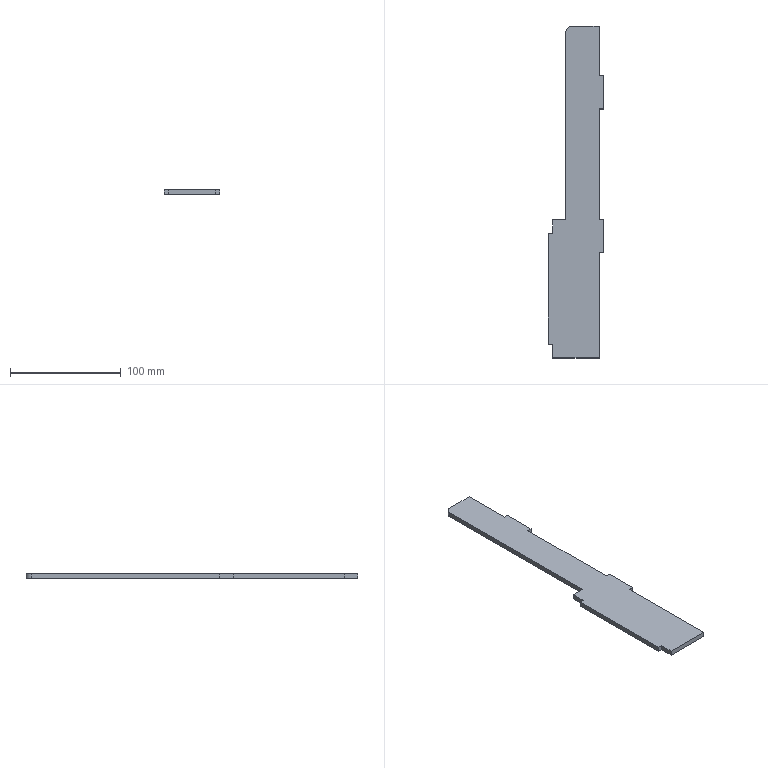Part | SolidWorks | features FlatPattern 1, SMBaseFlange 1, SheetMetal 1 | 1 solid | 21 faces | box 49.8 x 300 x 4.5 mm | volume 49993 mm3 | plane 20 | cylinder 1 | commonest cylinder face diameters 10 x1
STEP:
#1=CARTESIAN_POINT('',(-1112.571,288.492,0.));
#2=VERTEX_POINT('',#1);
#3=CARTESIAN_POINT('',(-1112.571,333.492,0.));
#4=VERTEX_POINT('',#3);
#5=CARTESIAN_POINT('',(-1112.571,288.492,0.));
#6=DIRECTION('',(0.,1.,0.));
#7=VECTOR('',#6,1000.);
#8=LINE('',#5,#7);
#9=EDGE_CURVE('',#2,#4,#8,.T.);
#10=ORIENTED_EDGE('',*,*,#9,.F.);
#11=CARTESIAN_POINT('',(-1112.571,288.492,-4.5));
#12=VERTEX_POINT('',#11);
#13=CARTESIAN_POINT('',(-1112.571,288.492,-4.5));
#14=DIRECTION('',(0.,0.,1.));
#15=VECTOR('',#14,1000.);
#16=LINE('',#13,#15);
#17=EDGE_CURVE('',#12,#2,#16,.T.);
#18=ORIENTED_EDGE('',*,*,#17,.F.);
#19=CARTESIAN_POINT('',(-1112.571,333.492,-4.5));
#20=VERTEX_POINT('',#19);
#21=CARTESIAN_POINT('',(-1112.571,288.492,-4.5));
#22=DIRECTION('',(0.,1.,0.));
#23=VECTOR('',#22,1000.);
#24=LINE('',#21,#23);
#25=EDGE_CURVE('',#12,#20,#24,.T.);
#26=ORIENTED_EDGE('',*,*,#25,.T.);
#27=CARTESIAN_POINT('',(-1112.571,333.492,-4.5));
#28=DIRECTION('',(0.,0.,1.));
#29=VECTOR('',#28,1000.);
#30=LINE('',#27,#29);
#31=EDGE_CURVE('',#20,#4,#30,.T.);
#32=ORIENTED_EDGE('',*,*,#31,.T.);
#33=EDGE_LOOP('',(#10,#18,#26,#32));
#34=FACE_OUTER_BOUND('',#33,.T.);
#35=CARTESIAN_POINT('',(-1112.571,288.492,-4.5));
#36=DIRECTION('',(1.,0.,0.));
#37=DIRECTION('',(0.,0.,-1.));
#38=AXIS2_PLACEMENT_3D('',#35,#36,#37);
#39=PLANE('',#38);
#40=ADVANCED_FACE('',(#34),#39,.T.);
#41=CARTESIAN_POINT('',(-1108.571,288.492,0.));
#42=VERTEX_POINT('',#41);
#43=CARTESIAN_POINT('',(-1108.571,288.492,0.));
#44=DIRECTION('',(-1.,0.,0.));
#45=VECTOR('',#44,1000.);
#46=LINE('',#43,#45);
#47=EDGE_CURVE('',#42,#2,#46,.T.);
#48=ORIENTED_EDGE('',*,*,#47,.F.);
#49=CARTESIAN_POINT('',(-1108.571,288.492,-4.5));
#50=VERTEX_POINT('',#49);
#51=CARTESIAN_POINT('',(-1108.571,288.492,-4.5));
#52=DIRECTION('',(0.,0.,1.));
#53=VECTOR('',#52,1000.);
#54=LINE('',#51,#53);
#55=EDGE_CURVE('',#50,#42,#54,.T.);
#56=ORIENTED_EDGE('',*,*,#55,.F.);
#57=CARTESIAN_POINT('',(-1108.571,288.492,-4.5));
#58=DIRECTION('',(-1.,0.,0.));
#59=VECTOR('',#58,1000.);
#60=LINE('',#57,#59);
#61=EDGE_CURVE('',#50,#12,#60,.T.);
#62=ORIENTED_EDGE('',*,*,#61,.T.);
#63=ORIENTED_EDGE('',*,*,#17,.T.);
#64=EDGE_LOOP('',(#48,#56,#62,#63));
#65=FACE_OUTER_BOUND('',#64,.T.);
#66=CARTESIAN_POINT('',(-1108.571,288.492,-4.5));
#67=DIRECTION('',(0.,1.,0.));
#68=DIRECTION('',(0.,0.,1.));
#69=AXIS2_PLACEMENT_3D('',#66,#67,#68);
#70=PLANE('',#69);
#71=ADVANCED_FACE('',(#65),#70,.T.);
#72=CARTESIAN_POINT('',(-1108.571,258.492,0.));
#73=VERTEX_POINT('',#72);
#74=CARTESIAN_POINT('',(-1108.571,258.492,0.));
#75=DIRECTION('',(0.,1.,0.));
#76=VECTOR('',#75,1000.);
#77=LINE('',#74,#76);
#78=EDGE_CURVE('',#73,#42,#77,.T.);
#79=ORIENTED_EDGE('',*,*,#78,.F.);
#80=CARTESIAN_POINT('',(-1108.571,258.492,-4.5));
#81=VERTEX_POINT('',#80);
#82=CARTESIAN_POINT('',(-1108.571,258.492,-4.5));
#83=DIRECTION('',(0.,0.,1.));
#84=VECTOR('',#83,1000.);
#85=LINE('',#82,#84);
#86=EDGE_CURVE('',#81,#73,#85,.T.);
#87=ORIENTED_EDGE('',*,*,#86,.F.);
#88=CARTESIAN_POINT('',(-1108.571,258.492,-4.5));
#89=DIRECTION('',(0.,1.,0.));
#90=VECTOR('',#89,1000.);
#91=LINE('',#88,#90);
#92=EDGE_CURVE('',#81,#50,#91,.T.);
#93=ORIENTED_EDGE('',*,*,#92,.T.);
#94=ORIENTED_EDGE('',*,*,#55,.T.);
#95=EDGE_LOOP('',(#79,#87,#93,#94));
#96=FACE_OUTER_BOUND('',#95,.T.);
#97=CARTESIAN_POINT('',(-1108.571,258.492,-4.5));
#98=DIRECTION('',(1.,0.,0.));
#99=DIRECTION('',(0.,0.,-1.));
#100=AXIS2_PLACEMENT_3D('',#97,#98,#99);
#101=PLANE('',#100);
#102=ADVANCED_FACE('',(#96),#101,.T.);
#103=CARTESIAN_POINT('',(-1112.571,258.492,0.));
#104=VERTEX_POINT('',#103);
#105=CARTESIAN_POINT('',(-1112.571,258.492,0.));
#106=DIRECTION('',(1.,0.,0.));
#107=VECTOR('',#106,1000.);
#108=LINE('',#105,#107);
#109=EDGE_CURVE('',#104,#73,#108,.T.);
#110=ORIENTED_EDGE('',*,*,#109,.F.);
#111=CARTESIAN_POINT('',(-1112.571,258.492,-4.5));
#112=VERTEX_POINT('',#111);
#113=CARTESIAN_POINT('',(-1112.571,258.492,-4.5));
#114=DIRECTION('',(0.,0.,1.));
#115=VECTOR('',#114,1000.);
#116=LINE('',#113,#115);
#117=EDGE_CURVE('',#112,#104,#116,.T.);
#118=ORIENTED_EDGE('',*,*,#117,.F.);
#119=CARTESIAN_POINT('',(-1112.571,258.492,-4.5));
#120=DIRECTION('',(1.,0.,0.));
#121=VECTOR('',#120,1000.);
#122=LINE('',#119,#121);
#123=EDGE_CURVE('',#112,#81,#122,.T.);
#124=ORIENTED_EDGE('',*,*,#123,.T.);
#125=ORIENTED_EDGE('',*,*,#86,.T.);
#126=EDGE_LOOP('',(#110,#118,#124,#125));
#127=FACE_OUTER_BOUND('',#126,.T.);
#128=CARTESIAN_POINT('',(-1112.571,258.492,-4.5));
#129=DIRECTION('',(0.,-1.,0.));
#130=DIRECTION('',(0.,0.,-1.));
#131=AXIS2_PLACEMENT_3D('',#128,#129,#130);
#132=PLANE('',#131);
#133=ADVANCED_FACE('',(#127),#132,.T.);
#134=CARTESIAN_POINT('',(-1112.571,158.492,0.));
#135=VERTEX_POINT('',#134);
#136=CARTESIAN_POINT('',(-1112.571,158.492,0.));
#137=DIRECTION('',(0.,1.,0.));
#138=VECTOR('',#137,1000.);
#139=LINE('',#136,#138);
#140=EDGE_CURVE('',#135,#104,#139,.T.);
#141=ORIENTED_EDGE('',*,*,#140,.F.);
#142=CARTESIAN_POINT('',(-1112.571,158.492,-4.5));
#143=VERTEX_POINT('',#142);
#144=CARTESIAN_POINT('',(-1112.571,158.492,-4.5));
#145=DIRECTION('',(0.,0.,1.));
#146=VECTOR('',#145,1000.);
#147=LINE('',#144,#146);
#148=EDGE_CURVE('',#143,#135,#147,.T.);
#149=ORIENTED_EDGE('',*,*,#148,.F.);
#150=CARTESIAN_POINT('',(-1112.571,158.492,-4.5));
#151=DIRECTION('',(0.,1.,0.));
#152=VECTOR('',#151,1000.);
#153=LINE('',#150,#152);
#154=EDGE_CURVE('',#143,#112,#153,.T.);
#155=ORIENTED_EDGE('',*,*,#154,.T.);
#156=ORIENTED_EDGE('',*,*,#117,.T.);
#157=EDGE_LOOP('',(#141,#149,#155,#156));
#158=FACE_OUTER_BOUND('',#157,.T.);
#159=CARTESIAN_POINT('',(-1112.571,158.492,-4.5));
#160=DIRECTION('',(1.,0.,0.));
#161=DIRECTION('',(0.,0.,-1.));
#162=AXIS2_PLACEMENT_3D('',#159,#160,#161);
#163=PLANE('',#162);
#164=ADVANCED_FACE('',(#158),#163,.T.);
#165=CARTESIAN_POINT('',(-1108.571,158.492,0.));
#166=VERTEX_POINT('',#165);
#167=CARTESIAN_POINT('',(-1108.571,158.492,0.));
#168=DIRECTION('',(-1.,0.,0.));
#169=VECTOR('',#168,1000.);
#170=LINE('',#167,#169);
#171=EDGE_CURVE('',#166,#135,#170,.T.);
#172=ORIENTED_EDGE('',*,*,#171,.F.);
#173=CARTESIAN_POINT('',(-1108.571,158.492,-4.5));
#174=VERTEX_POINT('',#173);
#175=CARTESIAN_POINT('',(-1108.571,158.492,-4.5));
#176=DIRECTION('',(0.,0.,1.));
#177=VECTOR('',#176,1000.);
#178=LINE('',#175,#177);
#179=EDGE_CURVE('',#174,#166,#178,.T.);
#180=ORIENTED_EDGE('',*,*,#179,.F.);
#181=CARTESIAN_POINT('',(-1108.571,158.492,-4.5));
#182=DIRECTION('',(-1.,0.,0.));
#183=VECTOR('',#182,1000.);
#184=LINE('',#181,#183);
#185=EDGE_CURVE('',#174,#143,#184,.T.);
#186=ORIENTED_EDGE('',*,*,#185,.T.);
#187=ORIENTED_EDGE('',*,*,#148,.T.);
#188=EDGE_LOOP('',(#172,#180,#186,#187));
#189=FACE_OUTER_BOUND('',#188,.T.);
#190=CARTESIAN_POINT('',(-1108.571,158.492,-4.5));
#191=DIRECTION('',(0.,1.,0.));
#192=DIRECTION('',(0.,0.,1.));
#193=AXIS2_PLACEMENT_3D('',#190,#191,#192);
#194=PLANE('',#193);
#195=ADVANCED_FACE('',(#189),#194,.T.);
#196=CARTESIAN_POINT('',(-1108.571,128.492,0.));
#197=VERTEX_POINT('',#196);
#198=CARTESIAN_POINT('',(-1108.571,128.492,0.));
#199=DIRECTION('',(0.,1.,0.));
#200=VECTOR('',#199,1000.);
#201=LINE('',#198,#200);
#202=EDGE_CURVE('',#197,#166,#201,.T.);
#203=ORIENTED_EDGE('',*,*,#202,.F.);
#204=CARTESIAN_POINT('',(-1108.571,128.492,-4.5));
#205=VERTEX_POINT('',#204);
#206=CARTESIAN_POINT('',(-1108.571,128.492,-4.5));
#207=DIRECTION('',(0.,0.,1.));
#208=VECTOR('',#207,1000.);
#209=LINE('',#206,#208);
#210=EDGE_CURVE('',#205,#197,#209,.T.);
#211=ORIENTED_EDGE('',*,*,#210,.F.);
#212=CARTESIAN_POINT('',(-1108.571,128.492,-4.5));
#213=DIRECTION('',(0.,1.,0.));
#214=VECTOR('',#213,1000.);
#215=LINE('',#212,#214);
#216=EDGE_CURVE('',#205,#174,#215,.T.);
#217=ORIENTED_EDGE('',*,*,#216,.T.);
#218=ORIENTED_EDGE('',*,*,#179,.T.);
#219=EDGE_LOOP('',(#203,#211,#217,#218));
#220=FACE_OUTER_BOUND('',#219,.T.);
#221=CARTESIAN_POINT('',(-1108.571,128.492,-4.5));
#222=DIRECTION('',(1.,0.,0.));
#223=DIRECTION('',(0.,0.,-1.));
#224=AXIS2_PLACEMENT_3D('',#221,#222,#223);
#225=PLANE('',#224);
#226=ADVANCED_FACE('',(#220),#225,.T.);
#227=CARTESIAN_POINT('',(-1112.571,128.492,0.));
#228=VERTEX_POINT('',#227);
#229=CARTESIAN_POINT('',(-1112.571,128.492,0.));
#230=DIRECTION('',(1.,0.,0.));
#231=VECTOR('',#230,1000.);
#232=LINE('',#229,#231);
#233=EDGE_CURVE('',#228,#197,#232,.T.);
#234=ORIENTED_EDGE('',*,*,#233,.F.);
#235=CARTESIAN_POINT('',(-1112.571,128.492,-4.5));
#236=VERTEX_POINT('',#235);
#237=CARTESIAN_POINT('',(-1112.571,128.492,-4.5));
#238=DIRECTION('',(0.,0.,1.));
#239=VECTOR('',#238,1000.);
#240=LINE('',#237,#239);
#241=EDGE_CURVE('',#236,#228,#240,.T.);
#242=ORIENTED_EDGE('',*,*,#241,.F.);
#243=CARTESIAN_POINT('',(-1112.571,128.492,-4.5));
#244=DIRECTION('',(1.,0.,0.));
#245=VECTOR('',#244,1000.);
#246=LINE('',#243,#245);
#247=EDGE_CURVE('',#236,#205,#246,.T.);
#248=ORIENTED_EDGE('',*,*,#247,.T.);
#249=ORIENTED_EDGE('',*,*,#210,.T.);
#250=EDGE_LOOP('',(#234,#242,#248,#249));
#251=FACE_OUTER_BOUND('',#250,.T.);
#252=CARTESIAN_POINT('',(-1112.571,128.492,-4.5));
#253=DIRECTION('',(0.,-1.,0.));
#254=DIRECTION('',(0.,0.,-1.));
#255=AXIS2_PLACEMENT_3D('',#252,#253,#254);
#256=PLANE('',#255);
#257=ADVANCED_FACE('',(#251),#256,.T.);
#258=CARTESIAN_POINT('',(-1112.571,33.492,0.));
#259=VERTEX_POINT('',#258);
#260=CARTESIAN_POINT('',(-1112.571,33.492,0.));
#261=DIRECTION('',(0.,1.,0.));
#262=VECTOR('',#261,1000.);
#263=LINE('',#260,#262);
#264=EDGE_CURVE('',#259,#228,#263,.T.);
#265=ORIENTED_EDGE('',*,*,#264,.F.);
#266=CARTESIAN_POINT('',(-1112.571,33.492,-4.5));
#267=VERTEX_POINT('',#266);
#268=CARTESIAN_POINT('',(-1112.571,33.492,-4.5));
#269=DIRECTION('',(0.,0.,1.));
#270=VECTOR('',#269,1000.);
#271=LINE('',#268,#270);
#272=EDGE_CURVE('',#267,#259,#271,.T.);
#273=ORIENTED_EDGE('',*,*,#272,.F.);
#274=CARTESIAN_POINT('',(-1112.571,33.492,-4.5));
#275=DIRECTION('',(0.,1.,0.));
#276=VECTOR('',#275,1000.);
#277=LINE('',#274,#276);
#278=EDGE_CURVE('',#267,#236,#277,.T.);
#279=ORIENTED_EDGE('',*,*,#278,.T.);
#280=ORIENTED_EDGE('',*,*,#241,.T.);
#281=EDGE_LOOP('',(#265,#273,#279,#280));
#282=FACE_OUTER_BOUND('',#281,.T.);
#283=CARTESIAN_POINT('',(-1112.571,33.492,-4.5));
#284=DIRECTION('',(1.,0.,0.));
#285=DIRECTION('',(0.,0.,-1.));
#286=AXIS2_PLACEMENT_3D('',#283,#284,#285);
#287=PLANE('',#286);
#288=ADVANCED_FACE('',(#282),#287,.T.);
#289=CARTESIAN_POINT('',(-1154.371,33.492,0.));
#290=VERTEX_POINT('',#289);
#291=CARTESIAN_POINT('',(-1154.371,33.492,0.));
#292=DIRECTION('',(1.,0.,0.));
#293=VECTOR('',#292,1000.);
#294=LINE('',#291,#293);
#295=EDGE_CURVE('',#290,#259,#294,.T.);
#296=ORIENTED_EDGE('',*,*,#295,.F.);
#297=CARTESIAN_POINT('',(-1154.371,33.492,-4.5));
#298=VERTEX_POINT('',#297);
#299=CARTESIAN_POINT('',(-1154.371,33.492,-4.5));
#300=DIRECTION('',(0.,0.,1.));
#301=VECTOR('',#300,1000.);
#302=LINE('',#299,#301);
#303=EDGE_CURVE('',#298,#290,#302,.T.);
#304=ORIENTED_EDGE('',*,*,#303,.F.);
#305=CARTESIAN_POINT('',(-1154.371,33.492,-4.5));
#306=DIRECTION('',(1.,0.,0.));
#307=VECTOR('',#306,1000.);
#308=LINE('',#305,#307);
#309=EDGE_CURVE('',#298,#267,#308,.T.);
#310=ORIENTED_EDGE('',*,*,#309,.T.);
#311=ORIENTED_EDGE('',*,*,#272,.T.);
#312=EDGE_LOOP('',(#296,#304,#310,#311));
#313=FACE_OUTER_BOUND('',#312,.T.);
#314=CARTESIAN_POINT('',(-1154.371,33.492,-4.5));
#315=DIRECTION('',(0.,-1.,0.));
#316=DIRECTION('',(0.,0.,-1.));
#317=AXIS2_PLACEMENT_3D('',#314,#315,#316);
#318=PLANE('',#317);
#319=ADVANCED_FACE('',(#313),#318,.T.);
#320=CARTESIAN_POINT('',(-1154.371,45.992,0.));
#321=VERTEX_POINT('',#320);
#322=CARTESIAN_POINT('',(-1154.371,45.992,0.));
#323=DIRECTION('',(0.,-1.,0.));
#324=VECTOR('',#323,1000.);
#325=LINE('',#322,#324);
#326=EDGE_CURVE('',#321,#290,#325,.T.);
#327=ORIENTED_EDGE('',*,*,#326,.F.);
#328=CARTESIAN_POINT('',(-1154.371,45.992,-4.5));
#329=VERTEX_POINT('',#328);
#330=CARTESIAN_POINT('',(-1154.371,45.992,-4.5));
#331=DIRECTION('',(0.,0.,1.));
#332=VECTOR('',#331,1000.);
#333=LINE('',#330,#332);
#334=EDGE_CURVE('',#329,#321,#333,.T.);
#335=ORIENTED_EDGE('',*,*,#334,.F.);
#336=CARTESIAN_POINT('',(-1154.371,45.992,-4.5));
#337=DIRECTION('',(0.,-1.,0.));
#338=VECTOR('',#337,1000.);
#339=LINE('',#336,#338);
#340=EDGE_CURVE('',#329,#298,#339,.T.);
#341=ORIENTED_EDGE('',*,*,#340,.T.);
#342=ORIENTED_EDGE('',*,*,#303,.T.);
#343=EDGE_LOOP('',(#327,#335,#341,#342));
#344=FACE_OUTER_BOUND('',#343,.T.);
#345=CARTESIAN_POINT('',(-1154.371,45.992,-4.5));
#346=DIRECTION('',(-1.,0.,0.));
#347=DIRECTION('',(0.,0.,1.));
#348=AXIS2_PLACEMENT_3D('',#345,#346,#347);
#349=PLANE('',#348);
#350=ADVANCED_FACE('',(#344),#349,.T.);
#351=CARTESIAN_POINT('',(-1158.371,45.992,0.));
#352=VERTEX_POINT('',#351);
#353=CARTESIAN_POINT('',(-1154.371,45.992,0.));
#354=DIRECTION('',(1.,0.,0.));
#355=VECTOR('',#354,1000.);
#356=LINE('',#353,#355);
#357=EDGE_CURVE('',#352,#321,#356,.T.);
#358=ORIENTED_EDGE('',*,*,#357,.F.);
#359=CARTESIAN_POINT('',(-1158.371,45.992,-4.5));
#360=VERTEX_POINT('',#359);
#361=CARTESIAN_POINT('',(-1158.371,45.992,-4.5));
#362=DIRECTION('',(0.,0.,1.));
#363=VECTOR('',#362,1000.);
#364=LINE('',#361,#363);
#365=EDGE_CURVE('',#360,#352,#364,.T.);
#366=ORIENTED_EDGE('',*,*,#365,.F.);
#367=CARTESIAN_POINT('',(-1154.371,45.992,-4.5));
#368=DIRECTION('',(1.,0.,0.));
#369=VECTOR('',#368,1000.);
#370=LINE('',#367,#369);
#371=EDGE_CURVE('',#360,#329,#370,.T.);
#372=ORIENTED_EDGE('',*,*,#371,.T.);
#373=ORIENTED_EDGE('',*,*,#334,.T.);
#374=EDGE_LOOP('',(#358,#366,#372,#373));
#375=FACE_OUTER_BOUND('',#374,.T.);
#376=CARTESIAN_POINT('',(-1154.371,45.992,-4.5));
#377=DIRECTION('',(0.,-1.,0.));
#378=DIRECTION('',(0.,0.,-1.));
#379=AXIS2_PLACEMENT_3D('',#376,#377,#378);
#380=PLANE('',#379);
#381=ADVANCED_FACE('',(#375),#380,.T.);
#382=CARTESIAN_POINT('',(-1158.371,145.992,0.));
#383=VERTEX_POINT('',#382);
#384=CARTESIAN_POINT('',(-1158.371,45.992,0.));
#385=DIRECTION('',(0.,-1.,0.));
#386=VECTOR('',#385,1000.);
#387=LINE('',#384,#386);
#388=EDGE_CURVE('',#383,#352,#387,.T.);
#389=ORIENTED_EDGE('',*,*,#388,.F.);
#390=CARTESIAN_POINT('',(-1158.371,145.992,-4.5));
#391=VERTEX_POINT('',#390);
#392=CARTESIAN_POINT('',(-1158.371,145.992,-4.5));
#393=DIRECTION('',(0.,0.,1.));
#394=VECTOR('',#393,1000.);
#395=LINE('',#392,#394);
#396=EDGE_CURVE('',#391,#383,#395,.T.);
#397=ORIENTED_EDGE('',*,*,#396,.F.);
#398=CARTESIAN_POINT('',(-1158.371,45.992,-4.5));
#399=DIRECTION('',(0.,-1.,0.));
#400=VECTOR('',#399,1000.);
#401=LINE('',#398,#400);
#402=EDGE_CURVE('',#391,#360,#401,.T.);
#403=ORIENTED_EDGE('',*,*,#402,.T.);
#404=ORIENTED_EDGE('',*,*,#365,.T.);
#405=EDGE_LOOP('',(#389,#397,#403,#404));
#406=FACE_OUTER_BOUND('',#405,.T.);
#407=CARTESIAN_POINT('',(-1158.371,45.992,-4.5));
#408=DIRECTION('',(-1.,0.,0.));
#409=DIRECTION('',(0.,0.,1.));
#410=AXIS2_PLACEMENT_3D('',#407,#408,#409);
#411=PLANE('',#410);
#412=ADVANCED_FACE('',(#406),#411,.T.);
#413=CARTESIAN_POINT('',(-1154.371,145.992,0.));
#414=VERTEX_POINT('',#413);
#415=CARTESIAN_POINT('',(-1158.371,145.992,0.));
#416=DIRECTION('',(-1.,0.,0.));
#417=VECTOR('',#416,1000.);
#418=LINE('',#415,#417);
#419=EDGE_CURVE('',#414,#383,#418,.T.);
#420=ORIENTED_EDGE('',*,*,#419,.F.);
#421=CARTESIAN_POINT('',(-1154.371,145.992,-4.5));
#422=VERTEX_POINT('',#421);
#423=CARTESIAN_POINT('',(-1154.371,145.992,-4.5));
#424=DIRECTION('',(0.,0.,1.));
#425=VECTOR('',#424,1000.);
#426=LINE('',#423,#425);
#427=EDGE_CURVE('',#422,#414,#426,.T.);
#428=ORIENTED_EDGE('',*,*,#427,.F.);
#429=CARTESIAN_POINT('',(-1158.371,145.992,-4.5));
#430=DIRECTION('',(-1.,0.,0.));
#431=VECTOR('',#430,1000.);
#432=LINE('',#429,#431);
#433=EDGE_CURVE('',#422,#391,#432,.T.);
#434=ORIENTED_EDGE('',*,*,#433,.T.);
#435=ORIENTED_EDGE('',*,*,#396,.T.);
#436=EDGE_LOOP('',(#420,#428,#434,#435));
#437=FACE_OUTER_BOUND('',#436,.T.);
#438=CARTESIAN_POINT('',(-1158.371,145.992,-4.5));
#439=DIRECTION('',(0.,1.,0.));
#440=DIRECTION('',(0.,0.,1.));
#441=AXIS2_PLACEMENT_3D('',#438,#439,#440);
#442=PLANE('',#441);
#443=ADVANCED_FACE('',(#437),#442,.T.);
#444=CARTESIAN_POINT('',(-1154.371,158.492,0.));
#445=VERTEX_POINT('',#444);
#446=CARTESIAN_POINT('',(-1154.371,158.492,0.));
#447=DIRECTION('',(0.,-1.,0.));
#448=VECTOR('',#447,1000.);
#449=LINE('',#446,#448);
#450=EDGE_CURVE('',#445,#414,#449,.T.);
#451=ORIENTED_EDGE('',*,*,#450,.F.);
#452=CARTESIAN_POINT('',(-1154.371,158.492,-4.5));
#453=VERTEX_POINT('',#452);
#454=CARTESIAN_POINT('',(-1154.371,158.492,-4.5));
#455=DIRECTION('',(0.,0.,1.));
#456=VECTOR('',#455,1000.);
#457=LINE('',#454,#456);
#458=EDGE_CURVE('',#453,#445,#457,.T.);
#459=ORIENTED_EDGE('',*,*,#458,.F.);
#460=CARTESIAN_POINT('',(-1154.371,158.492,-4.5));
#461=DIRECTION('',(0.,-1.,0.));
#462=VECTOR('',#461,1000.);
#463=LINE('',#460,#462);
#464=EDGE_CURVE('',#453,#422,#463,.T.);
#465=ORIENTED_EDGE('',*,*,#464,.T.);
#466=ORIENTED_EDGE('',*,*,#427,.T.);
#467=EDGE_LOOP('',(#451,#459,#465,#466));
#468=FACE_OUTER_BOUND('',#467,.T.);
#469=CARTESIAN_POINT('',(-1154.371,158.492,-4.5));
#470=DIRECTION('',(-1.,0.,0.));
#471=DIRECTION('',(0.,0.,1.));
#472=AXIS2_PLACEMENT_3D('',#469,#470,#471);
#473=PLANE('',#472);
#474=ADVANCED_FACE('',(#468),#473,.T.);
#475=CARTESIAN_POINT('',(-1142.571,158.492,0.));
#476=VERTEX_POINT('',#475);
#477=CARTESIAN_POINT('',(-1142.571,158.492,0.));
#478=DIRECTION('',(-1.,0.,0.));
#479=VECTOR('',#478,1000.);
#480=LINE('',#477,#479);
#481=EDGE_CURVE('',#476,#445,#480,.T.);
#482=ORIENTED_EDGE('',*,*,#481,.F.);
#483=CARTESIAN_POINT('',(-1142.571,158.492,-4.5));
#484=VERTEX_POINT('',#483);
#485=CARTESIAN_POINT('',(-1142.571,158.492,-4.5));
#486=DIRECTION('',(0.,0.,1.));
#487=VECTOR('',#486,1000.);
#488=LINE('',#485,#487);
#489=EDGE_CURVE('',#484,#476,#488,.T.);
#490=ORIENTED_EDGE('',*,*,#489,.F.);
#491=CARTESIAN_POINT('',(-1142.571,158.492,-4.5));
#492=DIRECTION('',(-1.,0.,0.));
#493=VECTOR('',#492,1000.);
#494=LINE('',#491,#493);
#495=EDGE_CURVE('',#484,#453,#494,.T.);
#496=ORIENTED_EDGE('',*,*,#495,.T.);
#497=ORIENTED_EDGE('',*,*,#458,.T.);
#498=EDGE_LOOP('',(#482,#490,#496,#497));
#499=FACE_OUTER_BOUND('',#498,.T.);
#500=CARTESIAN_POINT('',(-1142.571,158.492,-4.5));
#501=DIRECTION('',(0.,1.,0.));
#502=DIRECTION('',(0.,0.,1.));
#503=AXIS2_PLACEMENT_3D('',#500,#501,#502);
#504=PLANE('',#503);
#505=ADVANCED_FACE('',(#499),#504,.T.);
#506=CARTESIAN_POINT('',(-1142.571,328.492,0.));
#507=VERTEX_POINT('',#506);
#508=CARTESIAN_POINT('',(-1142.571,328.492,0.));
#509=DIRECTION('',(0.,-1.,0.));
#510=VECTOR('',#509,1000.);
#511=LINE('',#508,#510);
#512=EDGE_CURVE('',#507,#476,#511,.T.);
#513=ORIENTED_EDGE('',*,*,#512,.F.);
#514=CARTESIAN_POINT('',(-1142.571,328.492,-4.5));
#515=VERTEX_POINT('',#514);
#516=CARTESIAN_POINT('',(-1142.571,328.492,-4.5));
#517=DIRECTION('',(0.,0.,1.));
#518=VECTOR('',#517,1000.);
#519=LINE('',#516,#518);
#520=EDGE_CURVE('',#515,#507,#519,.T.);
#521=ORIENTED_EDGE('',*,*,#520,.F.);
#522=CARTESIAN_POINT('',(-1142.571,328.492,-4.5));
#523=DIRECTION('',(0.,-1.,0.));
#524=VECTOR('',#523,1000.);
#525=LINE('',#522,#524);
#526=EDGE_CURVE('',#515,#484,#525,.T.);
#527=ORIENTED_EDGE('',*,*,#526,.T.);
#528=ORIENTED_EDGE('',*,*,#489,.T.);
#529=EDGE_LOOP('',(#513,#521,#527,#528));
#530=FACE_OUTER_BOUND('',#529,.T.);
#531=CARTESIAN_POINT('',(-1142.571,328.492,-4.5));
#532=DIRECTION('',(-1.,0.,0.));
#533=DIRECTION('',(0.,0.,1.));
#534=AXIS2_PLACEMENT_3D('',#531,#532,#533);
#535=PLANE('',#534);
#536=ADVANCED_FACE('',(#530),#535,.T.);
#537=CARTESIAN_POINT('',(-1137.571,333.492,0.));
#538=VERTEX_POINT('',#537);
#539=CARTESIAN_POINT('',(-1137.571,328.492,0.));
#540=DIRECTION('',(0.,0.,1.));
#541=DIRECTION('',(1.,0.,0.));
#542=AXIS2_PLACEMENT_3D('',#539,#540,#541);
#543=CIRCLE('',#542,5.);
#544=EDGE_CURVE('',#538,#507,#543,.T.);
#545=ORIENTED_EDGE('',*,*,#544,.F.);
#546=CARTESIAN_POINT('',(-1137.571,333.492,-4.5));
#547=VERTEX_POINT('',#546);
#548=CARTESIAN_POINT('',(-1137.571,333.492,-4.5));
#549=DIRECTION('',(0.,0.,1.));
#550=VECTOR('',#549,1000.);
#551=LINE('',#548,#550);
#552=EDGE_CURVE('',#547,#538,#551,.T.);
#553=ORIENTED_EDGE('',*,*,#552,.F.);
#554=CARTESIAN_POINT('',(-1137.571,328.492,-4.5));
#555=DIRECTION('',(0.,0.,1.));
#556=DIRECTION('',(1.,0.,0.));
#557=AXIS2_PLACEMENT_3D('',#554,#555,#556);
#558=CIRCLE('',#557,5.);
#559=EDGE_CURVE('',#547,#515,#558,.T.);
#560=ORIENTED_EDGE('',*,*,#559,.T.);
#561=ORIENTED_EDGE('',*,*,#520,.T.);
#562=EDGE_LOOP('',(#545,#553,#560,#561));
#563=FACE_OUTER_BOUND('',#562,.T.);
#564=CARTESIAN_POINT('',(-1137.571,328.492,-4.5));
#565=DIRECTION('',(0.,0.,1.));
#566=DIRECTION('',(1.,0.,0.));
#567=AXIS2_PLACEMENT_3D('',#564,#565,#566);
#568=CYLINDRICAL_SURFACE('',#567,5.);
#569=ADVANCED_FACE('',(#563),#568,.T.);
#570=CARTESIAN_POINT('',(-1112.571,333.492,0.));
#571=DIRECTION('',(-1.,0.,0.));
#572=VECTOR('',#571,1000.);
#573=LINE('',#570,#572);
#574=EDGE_CURVE('',#4,#538,#573,.T.);
#575=ORIENTED_EDGE('',*,*,#574,.F.);
#576=ORIENTED_EDGE('',*,*,#31,.F.);
#577=CARTESIAN_POINT('',(-1112.571,333.492,-4.5));
#578=DIRECTION('',(-1.,0.,0.));
#579=VECTOR('',#578,1000.);
#580=LINE('',#577,#579);
#581=EDGE_CURVE('',#20,#547,#580,.T.);
#582=ORIENTED_EDGE('',*,*,#581,.T.);
#583=ORIENTED_EDGE('',*,*,#552,.T.);
#584=EDGE_LOOP('',(#575,#576,#582,#583));
#585=FACE_OUTER_BOUND('',#584,.T.);
#586=CARTESIAN_POINT('',(-1112.571,333.492,-4.5));
#587=DIRECTION('',(0.,1.,0.));
#588=DIRECTION('',(0.,0.,1.));
#589=AXIS2_PLACEMENT_3D('',#586,#587,#588);
#590=PLANE('',#589);
#591=ADVANCED_FACE('',(#585),#590,.T.);
#592=ORIENTED_EDGE('',*,*,#25,.F.);
#593=ORIENTED_EDGE('',*,*,#61,.F.);
#594=ORIENTED_EDGE('',*,*,#92,.F.);
#595=ORIENTED_EDGE('',*,*,#123,.F.);
#596=ORIENTED_EDGE('',*,*,#154,.F.);
#597=ORIENTED_EDGE('',*,*,#185,.F.);
#598=ORIENTED_EDGE('',*,*,#216,.F.);
#599=ORIENTED_EDGE('',*,*,#247,.F.);
#600=ORIENTED_EDGE('',*,*,#278,.F.);
#601=ORIENTED_EDGE('',*,*,#309,.F.);
#602=ORIENTED_EDGE('',*,*,#340,.F.);
#603=ORIENTED_EDGE('',*,*,#371,.F.);
#604=ORIENTED_EDGE('',*,*,#402,.F.);
#605=ORIENTED_EDGE('',*,*,#433,.F.);
#606=ORIENTED_EDGE('',*,*,#464,.F.);
#607=ORIENTED_EDGE('',*,*,#495,.F.);
#608=ORIENTED_EDGE('',*,*,#526,.F.);
#609=ORIENTED_EDGE('',*,*,#559,.F.);
#610=ORIENTED_EDGE('',*,*,#581,.F.);
#611=EDGE_LOOP('',(#592,#593,#594,#595,#596,#597,#598,#599,#600,#601,#602,#603,#604,#605,#606,#607,#608,#609,#610));
#612=FACE_OUTER_BOUND('',#611,.T.);
#613=CARTESIAN_POINT('',(-1137.571,328.492,-4.5));
#614=DIRECTION('',(0.,0.,1.));
#615=DIRECTION('',(1.,0.,0.));
#616=AXIS2_PLACEMENT_3D('',#613,#614,#615);
#617=PLANE('',#616);
#618=ADVANCED_FACE('',(#612),#617,.F.);
#619=ORIENTED_EDGE('',*,*,#9,.T.);
#620=ORIENTED_EDGE('',*,*,#574,.T.);
#621=ORIENTED_EDGE('',*,*,#544,.T.);
#622=ORIENTED_EDGE('',*,*,#512,.T.);
#623=ORIENTED_EDGE('',*,*,#481,.T.);
#624=ORIENTED_EDGE('',*,*,#450,.T.);
#625=ORIENTED_EDGE('',*,*,#419,.T.);
#626=ORIENTED_EDGE('',*,*,#388,.T.);
#627=ORIENTED_EDGE('',*,*,#357,.T.);
#628=ORIENTED_EDGE('',*,*,#326,.T.);
#629=ORIENTED_EDGE('',*,*,#295,.T.);
#630=ORIENTED_EDGE('',*,*,#264,.T.);
#631=ORIENTED_EDGE('',*,*,#233,.T.);
#632=ORIENTED_EDGE('',*,*,#202,.T.);
#633=ORIENTED_EDGE('',*,*,#171,.T.);
#634=ORIENTED_EDGE('',*,*,#140,.T.);
#635=ORIENTED_EDGE('',*,*,#109,.T.);
#636=ORIENTED_EDGE('',*,*,#78,.T.);
#637=ORIENTED_EDGE('',*,*,#47,.T.);
#638=EDGE_LOOP('',(#619,#620,#621,#622,#623,#624,#625,#626,#627,#628,#629,#630,#631,#632,#633,#634,#635,#636,#637));
#639=FACE_OUTER_BOUND('',#638,.T.);
#640=CARTESIAN_POINT('',(-1137.571,328.492,0.));
#641=DIRECTION('',(0.,0.,1.));
#642=DIRECTION('',(1.,0.,0.));
#643=AXIS2_PLACEMENT_3D('',#640,#641,#642);
#644=PLANE('',#643);
#645=ADVANCED_FACE('',(#639),#644,.T.);
#646=CLOSED_SHELL('',(#40,#71,#102,#133,#164,#195,#226,#257,#288,#319,#350,#381,#412,#443,#474,#505,#536,#569,#591,#618,#645));
#647=MANIFOLD_SOLID_BREP('',#646);
#648=CARTESIAN_POINT('',(0.,0.,0.));
#649=DIRECTION('',(0.,0.,1.));
#650=DIRECTION('',(1.,0.,0.));
#651=AXIS2_PLACEMENT_3D('',#648,#649,#650);
#652=(LENGTH_UNIT()NAMED_UNIT(*)SI_UNIT(.MILLI.,.METRE.));
#653=UNCERTAINTY_MEASURE_WITH_UNIT(LENGTH_MEASURE(0.00001),#652,'','');
#654=(NAMED_UNIT(*)PLANE_ANGLE_UNIT()SI_UNIT($,.RADIAN.));
#655=(NAMED_UNIT(*)SI_UNIT($,.STERADIAN.)SOLID_ANGLE_UNIT());
#656=(GEOMETRIC_REPRESENTATION_CONTEXT(3)GLOBAL_UNCERTAINTY_ASSIGNED_CONTEXT((#653))GLOBAL_UNIT_ASSIGNED_CONTEXT((#652,#654,#655))REPRESENTATION_CONTEXT('',''));
#657=ADVANCED_BREP_SHAPE_REPRESENTATION('',(#647,#651),#656);